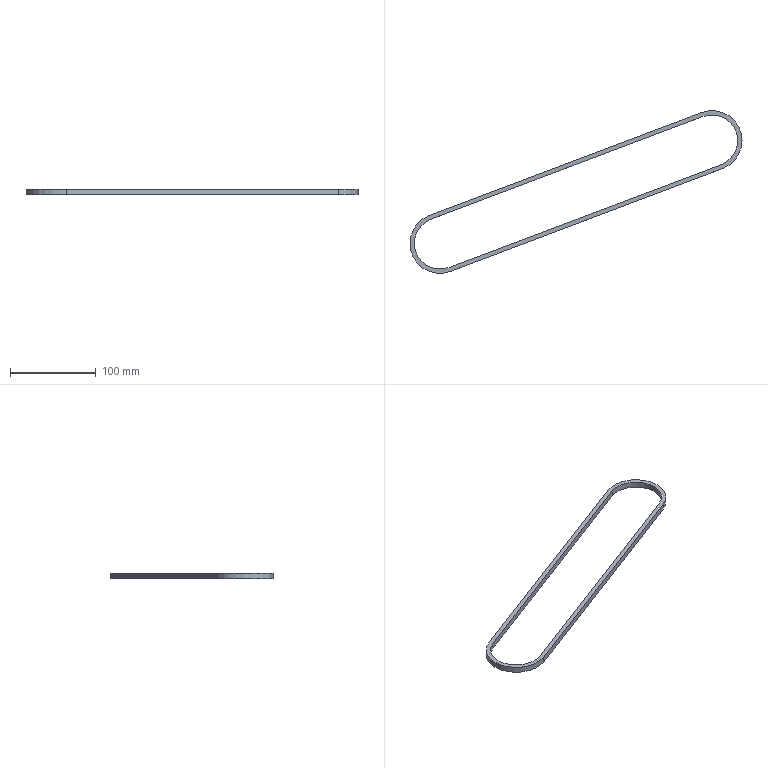Part | SolidWorks | 1 solid | 12 faces | box 388.198 x 190.208 x 7 mm | volume 30957 mm3 | cylinder 6 | plane 6 | commonest cylinder face diameters 60 x3 70 x3
STEP:
#1=CARTESIAN_POINT('',(-307.596,-148.272,179.));
#2=VERTEX_POINT('',#1);
#3=CARTESIAN_POINT('',(-328.8,-92.144,179.));
#4=VERTEX_POINT('',#3);
#5=CARTESIAN_POINT('',(-318.198,-120.208,179.));
#6=DIRECTION('',(0.,0.,-1.));
#7=DIRECTION('',(0.3534,-0.9355,0.));
#8=AXIS2_PLACEMENT_3D('',#5,#6,#7);
#9=CIRCLE('',#8,30.);
#10=EDGE_CURVE('',#2,#4,#9,.T.);
#11=ORIENTED_EDGE('',*,*,#10,.T.);
#12=CARTESIAN_POINT('',(-328.8,-92.144,186.));
#13=VERTEX_POINT('',#12);
#14=CARTESIAN_POINT('',(-328.8,-92.144,186.));
#15=DIRECTION('',(0.,0.,-1.));
#16=VECTOR('',#15,1000.);
#17=LINE('',#14,#16);
#18=EDGE_CURVE('',#13,#4,#17,.T.);
#19=ORIENTED_EDGE('',*,*,#18,.F.);
#20=CARTESIAN_POINT('',(-307.596,-148.272,186.));
#21=VERTEX_POINT('',#20);
#22=CARTESIAN_POINT('',(-318.198,-120.208,186.));
#23=DIRECTION('',(0.,0.,1.));
#24=DIRECTION('',(-0.3534,0.9355,0.));
#25=AXIS2_PLACEMENT_3D('',#22,#23,#24);
#26=CIRCLE('',#25,30.);
#27=EDGE_CURVE('',#13,#21,#26,.T.);
#28=ORIENTED_EDGE('',*,*,#27,.T.);
#29=CARTESIAN_POINT('',(-307.596,-148.272,179.));
#30=DIRECTION('',(0.,0.,1.));
#31=VECTOR('',#30,1000.);
#32=LINE('',#29,#31);
#33=EDGE_CURVE('',#2,#21,#32,.T.);
#34=ORIENTED_EDGE('',*,*,#33,.F.);
#35=EDGE_LOOP('',(#11,#19,#28,#34));
#36=FACE_OUTER_BOUND('',#35,.T.);
#37=CARTESIAN_POINT('',(-318.198,-120.208,186.));
#38=DIRECTION('',(0.,0.,1.));
#39=DIRECTION('',(1.,0.,0.));
#40=AXIS2_PLACEMENT_3D('',#37,#38,#39);
#41=CYLINDRICAL_SURFACE('',#40,30.);
#42=ADVANCED_FACE('',(#36),#41,.F.);
#43=CARTESIAN_POINT('',(-10.602,28.064,179.));
#44=VERTEX_POINT('',#43);
#45=CARTESIAN_POINT('',(-328.8,-92.144,179.));
#46=DIRECTION('',(0.9355,0.3534,0.));
#47=VECTOR('',#46,1000.);
#48=LINE('',#45,#47);
#49=EDGE_CURVE('',#4,#44,#48,.T.);
#50=ORIENTED_EDGE('',*,*,#49,.T.);
#51=CARTESIAN_POINT('',(-10.602,28.064,186.));
#52=VERTEX_POINT('',#51);
#53=CARTESIAN_POINT('',(-10.602,28.064,179.));
#54=DIRECTION('',(0.,0.,1.));
#55=VECTOR('',#54,1000.);
#56=LINE('',#53,#55);
#57=EDGE_CURVE('',#44,#52,#56,.T.);
#58=ORIENTED_EDGE('',*,*,#57,.T.);
#59=CARTESIAN_POINT('',(-10.602,28.064,186.));
#60=DIRECTION('',(-0.9355,-0.3534,0.));
#61=VECTOR('',#60,1000.);
#62=LINE('',#59,#61);
#63=EDGE_CURVE('',#52,#13,#62,.T.);
#64=ORIENTED_EDGE('',*,*,#63,.T.);
#65=ORIENTED_EDGE('',*,*,#18,.T.);
#66=EDGE_LOOP('',(#50,#58,#64,#65));
#67=FACE_OUTER_BOUND('',#66,.T.);
#68=CARTESIAN_POINT('',(-10.602,28.064,186.));
#69=DIRECTION('',(-0.3534,0.9355,0.));
#70=DIRECTION('',(0.,0.,1.));
#71=AXIS2_PLACEMENT_3D('',#68,#69,#70);
#72=PLANE('',#71);
#73=ADVANCED_FACE('',(#67),#72,.F.);
#74=CARTESIAN_POINT('',(10.602,-28.064,186.));
#75=VERTEX_POINT('',#74);
#76=CARTESIAN_POINT('',(-307.596,-148.272,186.));
#77=DIRECTION('',(0.9355,0.3534,0.));
#78=VECTOR('',#77,1000.);
#79=LINE('',#76,#78);
#80=EDGE_CURVE('',#21,#75,#79,.T.);
#81=ORIENTED_EDGE('',*,*,#80,.F.);
#82=ORIENTED_EDGE('',*,*,#27,.F.);
#83=ORIENTED_EDGE('',*,*,#63,.F.);
#84=CARTESIAN_POINT('',(30.,0.,186.));
#85=VERTEX_POINT('',#84);
#86=CARTESIAN_POINT('',(0.,0.,186.));
#87=DIRECTION('',(0.,0.,1.));
#88=DIRECTION('',(1.,0.,0.));
#89=AXIS2_PLACEMENT_3D('',#86,#87,#88);
#90=CIRCLE('',#89,30.);
#91=EDGE_CURVE('',#85,#52,#90,.T.);
#92=ORIENTED_EDGE('',*,*,#91,.F.);
#93=CARTESIAN_POINT('',(0.,0.,186.));
#94=DIRECTION('',(0.,0.,1.));
#95=DIRECTION('',(0.3534,-0.9355,0.));
#96=AXIS2_PLACEMENT_3D('',#93,#94,#95);
#97=CIRCLE('',#96,30.);
#98=EDGE_CURVE('',#75,#85,#97,.T.);
#99=ORIENTED_EDGE('',*,*,#98,.F.);
#100=EDGE_LOOP('',(#81,#82,#83,#92,#99));
#101=FACE_BOUND('',#100,.T.);
#102=CARTESIAN_POINT('',(35.,0.,186.));
#103=VERTEX_POINT('',#102);
#104=CARTESIAN_POINT('',(12.369,-32.742,186.));
#105=VERTEX_POINT('',#104);
#106=CARTESIAN_POINT('',(0.,0.,186.));
#107=DIRECTION('',(0.,0.,-1.));
#108=DIRECTION('',(1.,0.,0.));
#109=AXIS2_PLACEMENT_3D('',#106,#107,#108);
#110=CIRCLE('',#109,35.);
#111=EDGE_CURVE('',#103,#105,#110,.T.);
#112=ORIENTED_EDGE('',*,*,#111,.F.);
#113=CARTESIAN_POINT('',(-12.369,32.742,186.));
#114=VERTEX_POINT('',#113);
#115=CARTESIAN_POINT('',(0.,0.,186.));
#116=DIRECTION('',(0.,0.,-1.));
#117=DIRECTION('',(-0.3534,0.9355,0.));
#118=AXIS2_PLACEMENT_3D('',#115,#116,#117);
#119=CIRCLE('',#118,35.);
#120=EDGE_CURVE('',#114,#103,#119,.T.);
#121=ORIENTED_EDGE('',*,*,#120,.F.);
#122=CARTESIAN_POINT('',(-330.567,-87.467,186.));
#123=VERTEX_POINT('',#122);
#124=CARTESIAN_POINT('',(-330.567,-87.467,186.));
#125=DIRECTION('',(0.9355,0.3534,0.));
#126=VECTOR('',#125,1000.);
#127=LINE('',#124,#126);
#128=EDGE_CURVE('',#123,#114,#127,.T.);
#129=ORIENTED_EDGE('',*,*,#128,.F.);
#130=CARTESIAN_POINT('',(-305.829,-152.95,186.));
#131=VERTEX_POINT('',#130);
#132=CARTESIAN_POINT('',(-318.198,-120.208,186.));
#133=DIRECTION('',(0.,0.,-1.));
#134=DIRECTION('',(-1.,0.,0.));
#135=AXIS2_PLACEMENT_3D('',#132,#133,#134);
#136=CIRCLE('',#135,35.);
#137=EDGE_CURVE('',#131,#123,#136,.T.);
#138=ORIENTED_EDGE('',*,*,#137,.F.);
#139=CARTESIAN_POINT('',(12.369,-32.742,186.));
#140=DIRECTION('',(-0.9355,-0.3534,0.));
#141=VECTOR('',#140,1000.);
#142=LINE('',#139,#141);
#143=EDGE_CURVE('',#105,#131,#142,.T.);
#144=ORIENTED_EDGE('',*,*,#143,.F.);
#145=EDGE_LOOP('',(#112,#121,#129,#138,#144));
#146=FACE_OUTER_BOUND('',#145,.T.);
#147=CARTESIAN_POINT('',(-170.585,-29.701,186.));
#148=DIRECTION('',(0.,0.,1.));
#149=DIRECTION('',(1.,0.,0.));
#150=AXIS2_PLACEMENT_3D('',#147,#148,#149);
#151=PLANE('',#150);
#152=ADVANCED_FACE('',(#101,#146),#151,.T.);
#153=CARTESIAN_POINT('',(35.,0.,179.));
#154=VERTEX_POINT('',#153);
#155=CARTESIAN_POINT('',(35.,0.,186.));
#156=DIRECTION('',(0.,0.,-1.));
#157=VECTOR('',#156,1000.);
#158=LINE('',#155,#157);
#159=EDGE_CURVE('',#103,#154,#158,.T.);
#160=ORIENTED_EDGE('',*,*,#159,.F.);
#161=ORIENTED_EDGE('',*,*,#111,.T.);
#162=CARTESIAN_POINT('',(12.369,-32.742,179.));
#163=VERTEX_POINT('',#162);
#164=CARTESIAN_POINT('',(12.369,-32.742,179.));
#165=DIRECTION('',(0.,0.,1.));
#166=VECTOR('',#165,1000.);
#167=LINE('',#164,#166);
#168=EDGE_CURVE('',#163,#105,#167,.T.);
#169=ORIENTED_EDGE('',*,*,#168,.F.);
#170=CARTESIAN_POINT('',(0.,0.,179.));
#171=DIRECTION('',(0.,0.,1.));
#172=DIRECTION('',(0.3534,-0.9355,0.));
#173=AXIS2_PLACEMENT_3D('',#170,#171,#172);
#174=CIRCLE('',#173,35.);
#175=EDGE_CURVE('',#163,#154,#174,.T.);
#176=ORIENTED_EDGE('',*,*,#175,.T.);
#177=EDGE_LOOP('',(#160,#161,#169,#176));
#178=FACE_OUTER_BOUND('',#177,.T.);
#179=CARTESIAN_POINT('',(0.,0.,186.));
#180=DIRECTION('',(0.,0.,1.));
#181=DIRECTION('',(1.,0.,0.));
#182=AXIS2_PLACEMENT_3D('',#179,#180,#181);
#183=CYLINDRICAL_SURFACE('',#182,35.);
#184=ADVANCED_FACE('',(#178),#183,.T.);
#185=CARTESIAN_POINT('',(-12.369,32.742,179.));
#186=VERTEX_POINT('',#185);
#187=CARTESIAN_POINT('',(0.,0.,179.));
#188=DIRECTION('',(0.,0.,1.));
#189=DIRECTION('',(1.,0.,0.));
#190=AXIS2_PLACEMENT_3D('',#187,#188,#189);
#191=CIRCLE('',#190,35.);
#192=EDGE_CURVE('',#154,#186,#191,.T.);
#193=ORIENTED_EDGE('',*,*,#192,.T.);
#194=CARTESIAN_POINT('',(-12.369,32.742,186.));
#195=DIRECTION('',(0.,0.,-1.));
#196=VECTOR('',#195,1000.);
#197=LINE('',#194,#196);
#198=EDGE_CURVE('',#114,#186,#197,.T.);
#199=ORIENTED_EDGE('',*,*,#198,.F.);
#200=ORIENTED_EDGE('',*,*,#120,.T.);
#201=ORIENTED_EDGE('',*,*,#159,.T.);
#202=EDGE_LOOP('',(#193,#199,#200,#201));
#203=FACE_OUTER_BOUND('',#202,.T.);
#204=CARTESIAN_POINT('',(0.,0.,186.));
#205=DIRECTION('',(0.,0.,1.));
#206=DIRECTION('',(1.,0.,0.));
#207=AXIS2_PLACEMENT_3D('',#204,#205,#206);
#208=CYLINDRICAL_SURFACE('',#207,35.);
#209=ADVANCED_FACE('',(#203),#208,.T.);
#210=CARTESIAN_POINT('',(-330.567,-87.467,179.));
#211=VERTEX_POINT('',#210);
#212=CARTESIAN_POINT('',(-12.369,32.742,179.));
#213=DIRECTION('',(-0.9355,-0.3534,0.));
#214=VECTOR('',#213,1000.);
#215=LINE('',#212,#214);
#216=EDGE_CURVE('',#186,#211,#215,.T.);
#217=ORIENTED_EDGE('',*,*,#216,.T.);
#218=CARTESIAN_POINT('',(-330.567,-87.467,179.));
#219=DIRECTION('',(0.,0.,1.));
#220=VECTOR('',#219,1000.);
#221=LINE('',#218,#220);
#222=EDGE_CURVE('',#211,#123,#221,.T.);
#223=ORIENTED_EDGE('',*,*,#222,.T.);
#224=ORIENTED_EDGE('',*,*,#128,.T.);
#225=ORIENTED_EDGE('',*,*,#198,.T.);
#226=EDGE_LOOP('',(#217,#223,#224,#225));
#227=FACE_OUTER_BOUND('',#226,.T.);
#228=CARTESIAN_POINT('',(-12.369,32.742,186.));
#229=DIRECTION('',(-0.3534,0.9355,0.));
#230=DIRECTION('',(0.,0.,1.));
#231=AXIS2_PLACEMENT_3D('',#228,#229,#230);
#232=PLANE('',#231);
#233=ADVANCED_FACE('',(#227),#232,.T.);
#234=CARTESIAN_POINT('',(-305.829,-152.95,179.));
#235=VERTEX_POINT('',#234);
#236=CARTESIAN_POINT('',(-318.198,-120.208,179.));
#237=DIRECTION('',(0.,0.,1.));
#238=DIRECTION('',(-0.3534,0.9355,0.));
#239=AXIS2_PLACEMENT_3D('',#236,#237,#238);
#240=CIRCLE('',#239,35.);
#241=EDGE_CURVE('',#211,#235,#240,.T.);
#242=ORIENTED_EDGE('',*,*,#241,.T.);
#243=CARTESIAN_POINT('',(-305.829,-152.95,186.));
#244=DIRECTION('',(0.,0.,-1.));
#245=VECTOR('',#244,1000.);
#246=LINE('',#243,#245);
#247=EDGE_CURVE('',#131,#235,#246,.T.);
#248=ORIENTED_EDGE('',*,*,#247,.F.);
#249=ORIENTED_EDGE('',*,*,#137,.T.);
#250=ORIENTED_EDGE('',*,*,#222,.F.);
#251=EDGE_LOOP('',(#242,#248,#249,#250));
#252=FACE_OUTER_BOUND('',#251,.T.);
#253=CARTESIAN_POINT('',(-318.198,-120.208,186.));
#254=DIRECTION('',(0.,0.,1.));
#255=DIRECTION('',(1.,0.,0.));
#256=AXIS2_PLACEMENT_3D('',#253,#254,#255);
#257=CYLINDRICAL_SURFACE('',#256,35.);
#258=ADVANCED_FACE('',(#252),#257,.T.);
#259=CARTESIAN_POINT('',(-305.829,-152.95,179.));
#260=DIRECTION('',(0.9355,0.3534,0.));
#261=VECTOR('',#260,1000.);
#262=LINE('',#259,#261);
#263=EDGE_CURVE('',#235,#163,#262,.T.);
#264=ORIENTED_EDGE('',*,*,#263,.T.);
#265=ORIENTED_EDGE('',*,*,#168,.T.);
#266=ORIENTED_EDGE('',*,*,#143,.T.);
#267=ORIENTED_EDGE('',*,*,#247,.T.);
#268=EDGE_LOOP('',(#264,#265,#266,#267));
#269=FACE_OUTER_BOUND('',#268,.T.);
#270=CARTESIAN_POINT('',(-305.829,-152.95,186.));
#271=DIRECTION('',(0.3534,-0.9355,0.));
#272=DIRECTION('',(0.,0.,-1.));
#273=AXIS2_PLACEMENT_3D('',#270,#271,#272);
#274=PLANE('',#273);
#275=ADVANCED_FACE('',(#269),#274,.T.);
#276=CARTESIAN_POINT('',(30.,0.,179.));
#277=VERTEX_POINT('',#276);
#278=CARTESIAN_POINT('',(10.602,-28.064,179.));
#279=VERTEX_POINT('',#278);
#280=CARTESIAN_POINT('',(0.,0.,179.));
#281=DIRECTION('',(0.,0.,-1.));
#282=DIRECTION('',(1.,0.,0.));
#283=AXIS2_PLACEMENT_3D('',#280,#281,#282);
#284=CIRCLE('',#283,30.);
#285=EDGE_CURVE('',#277,#279,#284,.T.);
#286=ORIENTED_EDGE('',*,*,#285,.F.);
#287=CARTESIAN_POINT('',(0.,0.,179.));
#288=DIRECTION('',(0.,0.,-1.));
#289=DIRECTION('',(-0.3534,0.9355,0.));
#290=AXIS2_PLACEMENT_3D('',#287,#288,#289);
#291=CIRCLE('',#290,30.);
#292=EDGE_CURVE('',#44,#277,#291,.T.);
#293=ORIENTED_EDGE('',*,*,#292,.F.);
#294=ORIENTED_EDGE('',*,*,#49,.F.);
#295=ORIENTED_EDGE('',*,*,#10,.F.);
#296=CARTESIAN_POINT('',(10.602,-28.064,179.));
#297=DIRECTION('',(-0.9355,-0.3534,0.));
#298=VECTOR('',#297,1000.);
#299=LINE('',#296,#298);
#300=EDGE_CURVE('',#279,#2,#299,.T.);
#301=ORIENTED_EDGE('',*,*,#300,.F.);
#302=EDGE_LOOP('',(#286,#293,#294,#295,#301));
#303=FACE_BOUND('',#302,.T.);
#304=ORIENTED_EDGE('',*,*,#263,.F.);
#305=ORIENTED_EDGE('',*,*,#241,.F.);
#306=ORIENTED_EDGE('',*,*,#216,.F.);
#307=ORIENTED_EDGE('',*,*,#192,.F.);
#308=ORIENTED_EDGE('',*,*,#175,.F.);
#309=EDGE_LOOP('',(#304,#305,#306,#307,#308));
#310=FACE_OUTER_BOUND('',#309,.T.);
#311=CARTESIAN_POINT('',(-170.585,-29.701,179.));
#312=DIRECTION('',(0.,0.,1.));
#313=DIRECTION('',(1.,0.,0.));
#314=AXIS2_PLACEMENT_3D('',#311,#312,#313);
#315=PLANE('',#314);
#316=ADVANCED_FACE('',(#303,#310),#315,.F.);
#317=CARTESIAN_POINT('',(30.,0.,186.));
#318=DIRECTION('',(0.,0.,-1.));
#319=VECTOR('',#318,1000.);
#320=LINE('',#317,#319);
#321=EDGE_CURVE('',#85,#277,#320,.T.);
#322=ORIENTED_EDGE('',*,*,#321,.F.);
#323=ORIENTED_EDGE('',*,*,#91,.T.);
#324=ORIENTED_EDGE('',*,*,#57,.F.);
#325=ORIENTED_EDGE('',*,*,#292,.T.);
#326=EDGE_LOOP('',(#322,#323,#324,#325));
#327=FACE_OUTER_BOUND('',#326,.T.);
#328=CARTESIAN_POINT('',(0.,0.,186.));
#329=DIRECTION('',(0.,0.,1.));
#330=DIRECTION('',(1.,0.,0.));
#331=AXIS2_PLACEMENT_3D('',#328,#329,#330);
#332=CYLINDRICAL_SURFACE('',#331,30.);
#333=ADVANCED_FACE('',(#327),#332,.F.);
#334=ORIENTED_EDGE('',*,*,#285,.T.);
#335=CARTESIAN_POINT('',(10.602,-28.064,186.));
#336=DIRECTION('',(0.,0.,-1.));
#337=VECTOR('',#336,1000.);
#338=LINE('',#335,#337);
#339=EDGE_CURVE('',#75,#279,#338,.T.);
#340=ORIENTED_EDGE('',*,*,#339,.F.);
#341=ORIENTED_EDGE('',*,*,#98,.T.);
#342=ORIENTED_EDGE('',*,*,#321,.T.);
#343=EDGE_LOOP('',(#334,#340,#341,#342));
#344=FACE_OUTER_BOUND('',#343,.T.);
#345=CARTESIAN_POINT('',(0.,0.,186.));
#346=DIRECTION('',(0.,0.,1.));
#347=DIRECTION('',(1.,0.,0.));
#348=AXIS2_PLACEMENT_3D('',#345,#346,#347);
#349=CYLINDRICAL_SURFACE('',#348,30.);
#350=ADVANCED_FACE('',(#344),#349,.F.);
#351=ORIENTED_EDGE('',*,*,#300,.T.);
#352=ORIENTED_EDGE('',*,*,#33,.T.);
#353=ORIENTED_EDGE('',*,*,#80,.T.);
#354=ORIENTED_EDGE('',*,*,#339,.T.);
#355=EDGE_LOOP('',(#351,#352,#353,#354));
#356=FACE_OUTER_BOUND('',#355,.T.);
#357=CARTESIAN_POINT('',(-307.596,-148.272,186.));
#358=DIRECTION('',(0.3534,-0.9355,0.));
#359=DIRECTION('',(0.,0.,-1.));
#360=AXIS2_PLACEMENT_3D('',#357,#358,#359);
#361=PLANE('',#360);
#362=ADVANCED_FACE('',(#356),#361,.F.);
#363=CLOSED_SHELL('',(#42,#73,#152,#184,#209,#233,#258,#275,#316,#333,#350,#362));
#364=MANIFOLD_SOLID_BREP('',#363);
#365=CARTESIAN_POINT('',(0.,0.,0.));
#366=DIRECTION('',(0.,0.,1.));
#367=DIRECTION('',(1.,0.,0.));
#368=AXIS2_PLACEMENT_3D('',#365,#366,#367);
#369=(LENGTH_UNIT()NAMED_UNIT(*)SI_UNIT(.MILLI.,.METRE.));
#370=UNCERTAINTY_MEASURE_WITH_UNIT(LENGTH_MEASURE(0.00001),#369,'','');
#371=(NAMED_UNIT(*)PLANE_ANGLE_UNIT()SI_UNIT($,.RADIAN.));
#372=(NAMED_UNIT(*)SI_UNIT($,.STERADIAN.)SOLID_ANGLE_UNIT());
#373=(GEOMETRIC_REPRESENTATION_CONTEXT(3)GLOBAL_UNCERTAINTY_ASSIGNED_CONTEXT((#370))GLOBAL_UNIT_ASSIGNED_CONTEXT((#369,#371,#372))REPRESENTATION_CONTEXT('',''));
#374=ADVANCED_BREP_SHAPE_REPRESENTATION('',(#364,#368),#373);